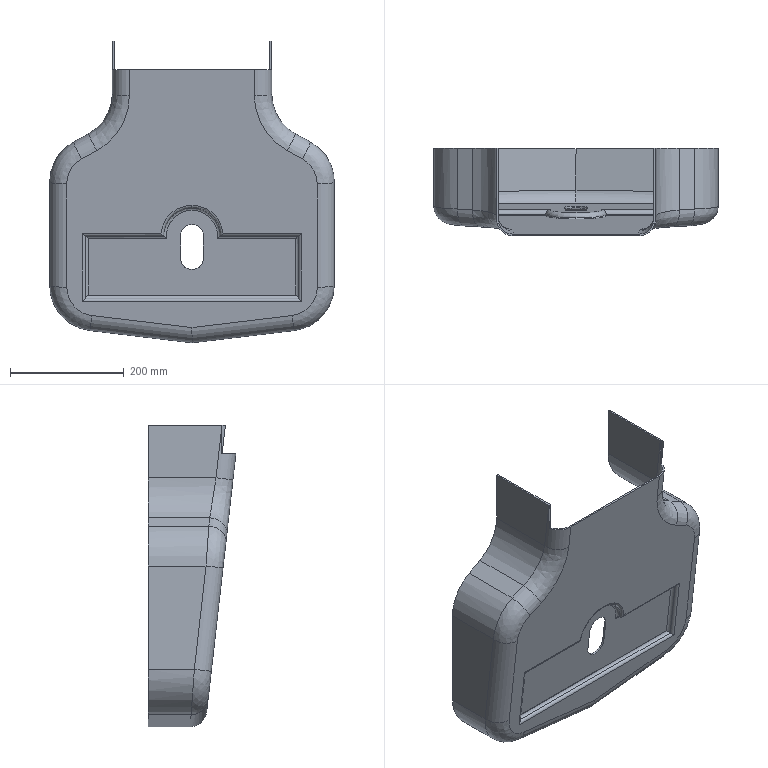Part | SolidWorks | 1 solid | 100 faces | box 500 x 154.34 x 530 mm | volume 1123560 mm3 | cylinder 53 | plane 29 | spline 12 | torus 6 | commonest cylinder face diameters 10 x11 54 x8 60 x8 16 x6 160 x6 4 x5